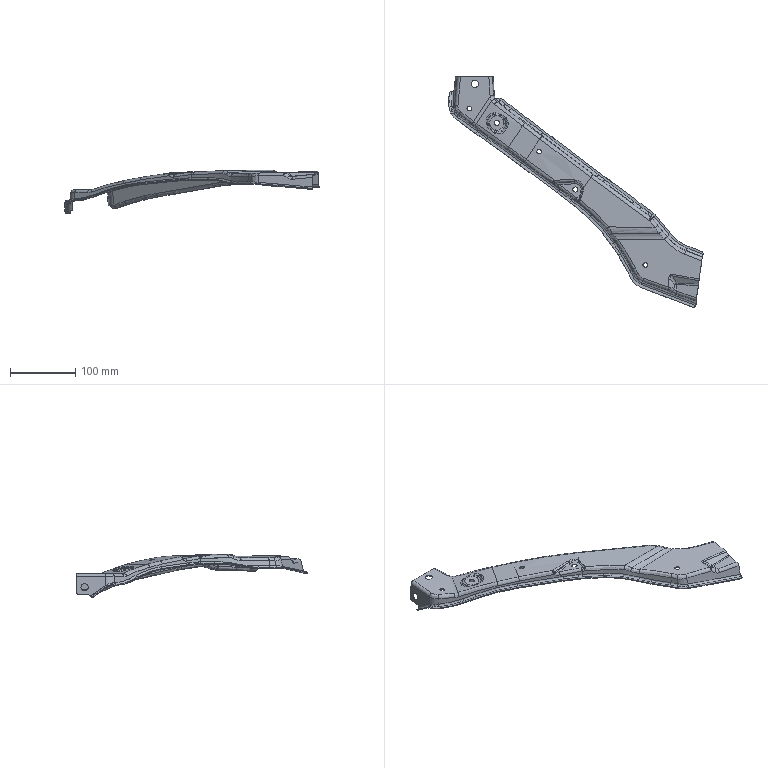Part | 1 solid | 418 faces | box 388.525 x 352.632 x 66.972 mm | volume 58362 mm3 | spline 299 | cylinder 97 | plane 18 | sphere 4 | commonest cylinder face diameters 10 x19 7.6 x15 8 x13 10.4 x7 6 x6 8.4 x6